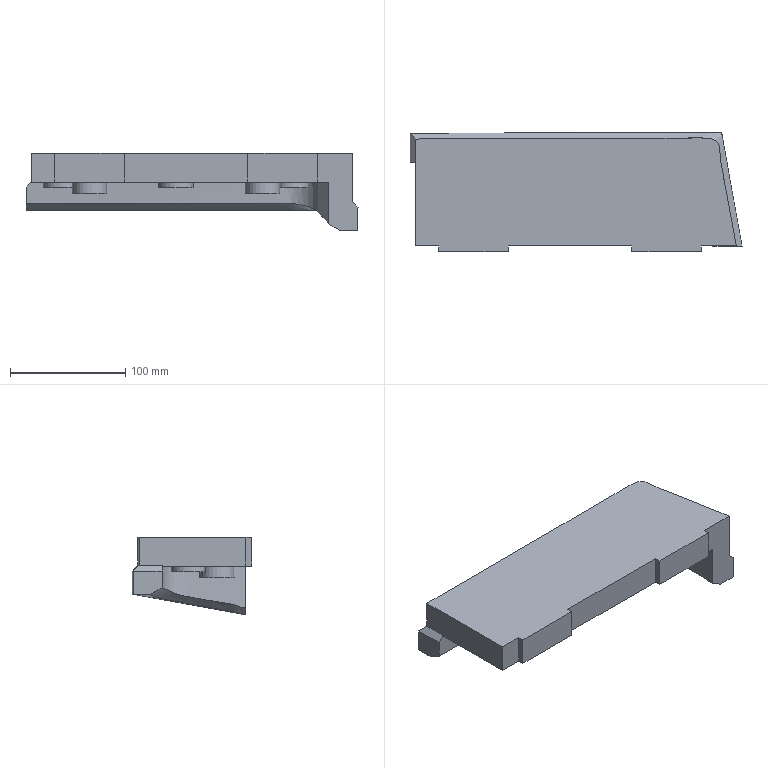Part | NX | features solid 2 | 1 solid | 32 faces | box 288.517 x 103.551 x 67.613 mm | volume 913973 mm3 | plane 20 | spline 7 | cylinder 5 | commonest cylinder face diameters 30 x5